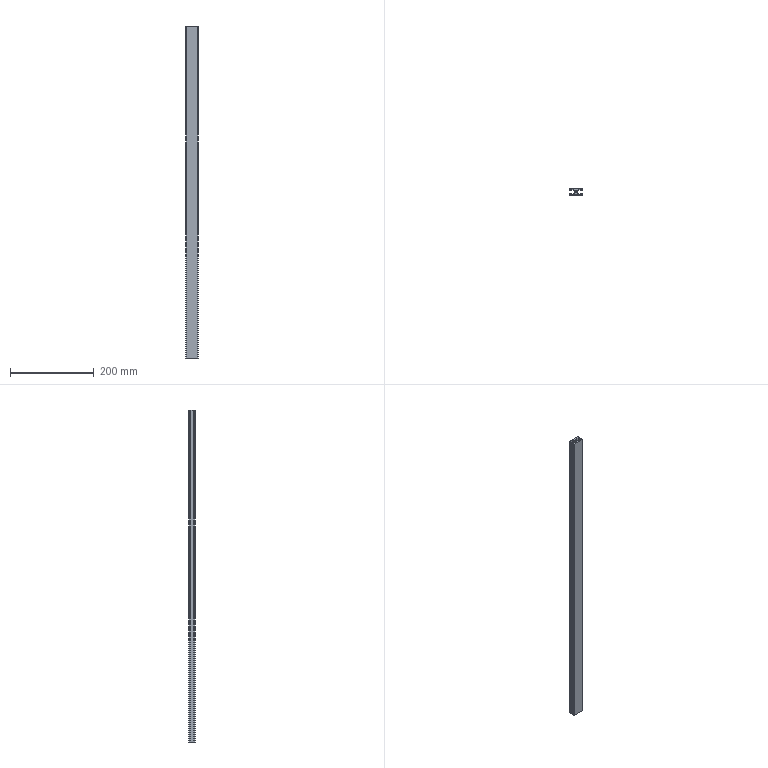Part | SolidWorks | features BaseBody 1, MoveFace 1 | 1 solid | 53 faces | box 30 x 15 x 791 mm | volume 190764 mm3 | plane 38 | cylinder 15 | commonest cylinder face diameters 1 x6 5 x5 2 x4